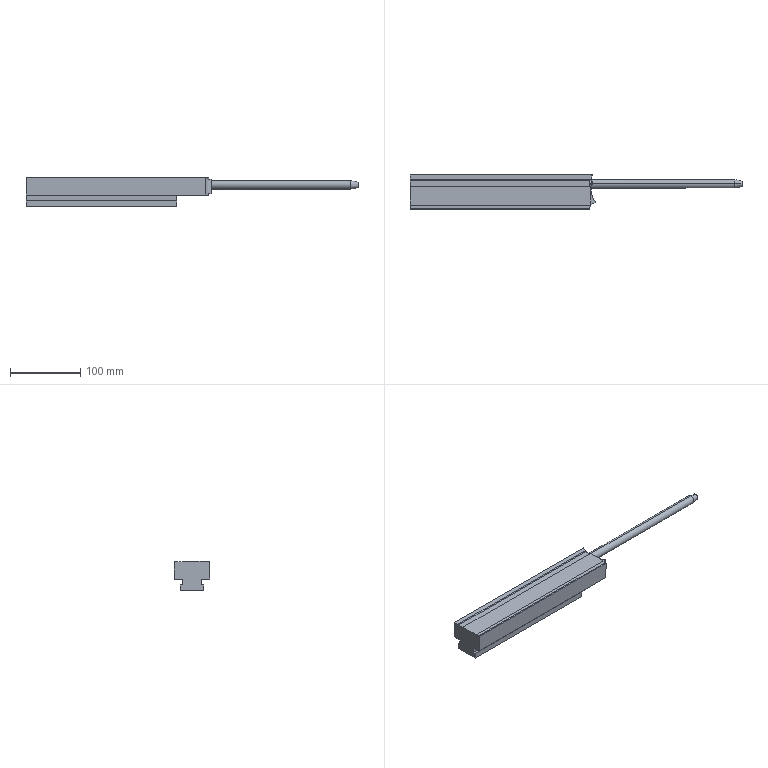Part | Creo | 1 solid | 51 faces | box 471.865 x 49.883 x 41.581 mm | volume 453906 mm3 | plane 27 | cylinder 19 | other 3 | cone 2 | commonest cylinder face diameters 12 x3 20.181 x3 16 x2 1.002 x1 22.141 x1 22.175 x1